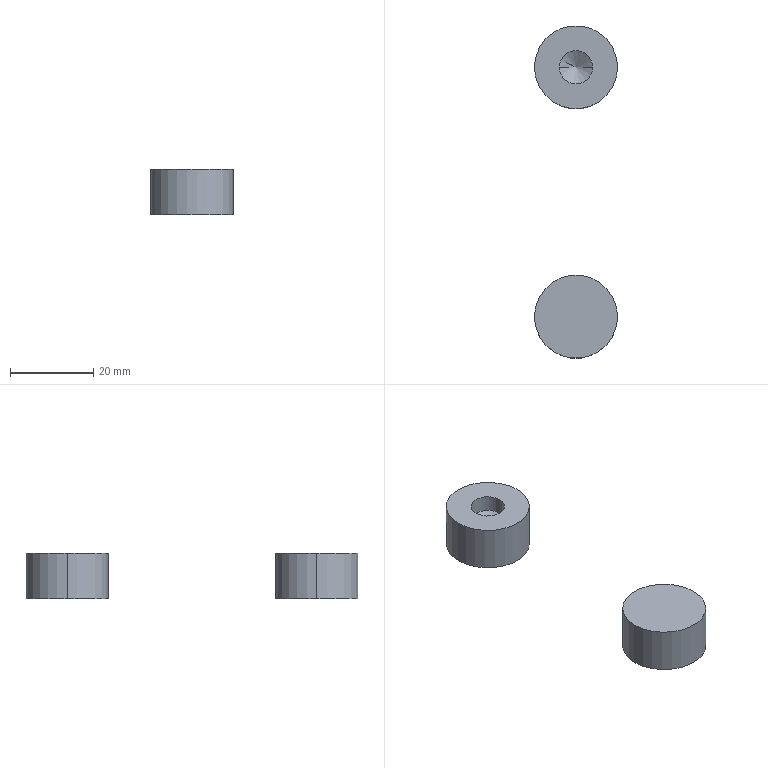Part | SolidWorks | features BaseBody 2 | 2 solids | 12 faces | box 20 x 80 x 11 mm | volume 6670 mm3 | cylinder 6 | plane 4 | cone 2 | commonest cylinder face diameters 20 x4 8 x2
STEP:
#1=CARTESIAN_POINT('',(70.,6.5,-439.5));
#2=VERTEX_POINT('',#1);
#3=CARTESIAN_POINT('',(50.,6.5,-439.5));
#4=VERTEX_POINT('',#3);
#5=CARTESIAN_POINT('',(60.,6.5,-439.5));
#6=DIRECTION('',(0.,0.,1.));
#7=DIRECTION('',(-1.,0.,0.));
#8=AXIS2_PLACEMENT_3D('',#5,#6,#7);
#9=CIRCLE('',#8,10.);
#10=EDGE_CURVE('',#2,#4,#9,.T.);
#11=ORIENTED_EDGE('',*,*,#10,.T.);
#12=CARTESIAN_POINT('',(50.,6.5,-428.5));
#13=VERTEX_POINT('',#12);
#14=CARTESIAN_POINT('',(50.,6.5,-439.5));
#15=DIRECTION('',(0.,0.,1.));
#16=VECTOR('',#15,1000.);
#17=LINE('',#14,#16);
#18=EDGE_CURVE('',#4,#13,#17,.T.);
#19=ORIENTED_EDGE('',*,*,#18,.T.);
#20=CARTESIAN_POINT('',(70.,6.5,-428.5));
#21=VERTEX_POINT('',#20);
#22=CARTESIAN_POINT('',(60.,6.5,-428.5));
#23=DIRECTION('',(0.,0.,1.));
#24=DIRECTION('',(-1.,0.,0.));
#25=AXIS2_PLACEMENT_3D('',#22,#23,#24);
#26=CIRCLE('',#25,10.);
#27=EDGE_CURVE('',#21,#13,#26,.T.);
#28=ORIENTED_EDGE('',*,*,#27,.F.);
#29=CARTESIAN_POINT('',(70.,6.5,-439.5));
#30=DIRECTION('',(0.,0.,1.));
#31=VECTOR('',#30,1000.);
#32=LINE('',#29,#31);
#33=EDGE_CURVE('',#2,#21,#32,.T.);
#34=ORIENTED_EDGE('',*,*,#33,.F.);
#35=EDGE_LOOP('',(#11,#19,#28,#34));
#36=FACE_OUTER_BOUND('',#35,.T.);
#37=CARTESIAN_POINT('',(60.,6.5,-439.5));
#38=DIRECTION('',(0.,0.,1.));
#39=DIRECTION('',(1.,0.,0.));
#40=AXIS2_PLACEMENT_3D('',#37,#38,#39);
#41=CYLINDRICAL_SURFACE('',#40,10.);
#42=ADVANCED_FACE('',(#36),#41,.T.);
#43=ORIENTED_EDGE('',*,*,#27,.T.);
#44=CARTESIAN_POINT('',(60.,6.5,-428.5));
#45=DIRECTION('',(0.,0.,1.));
#46=DIRECTION('',(-1.,0.,0.));
#47=AXIS2_PLACEMENT_3D('',#44,#45,#46);
#48=CIRCLE('',#47,10.);
#49=EDGE_CURVE('',#13,#21,#48,.T.);
#50=ORIENTED_EDGE('',*,*,#49,.T.);
#51=EDGE_LOOP('',(#43,#50));
#52=FACE_OUTER_BOUND('',#51,.T.);
#53=CARTESIAN_POINT('',(60.,6.5,-428.5));
#54=DIRECTION('',(0.,0.,-1.));
#55=DIRECTION('',(0.,-1.,0.));
#56=AXIS2_PLACEMENT_3D('',#53,#54,#55);
#57=PLANE('',#56);
#58=ADVANCED_FACE('',(#52),#57,.F.);
#59=ORIENTED_EDGE('',*,*,#10,.F.);
#60=CARTESIAN_POINT('',(60.,6.5,-439.5));
#61=DIRECTION('',(0.,0.,1.));
#62=DIRECTION('',(-1.,0.,0.));
#63=AXIS2_PLACEMENT_3D('',#60,#61,#62);
#64=CIRCLE('',#63,10.);
#65=EDGE_CURVE('',#4,#2,#64,.T.);
#66=ORIENTED_EDGE('',*,*,#65,.F.);
#67=EDGE_LOOP('',(#59,#66));
#68=FACE_OUTER_BOUND('',#67,.T.);
#69=CARTESIAN_POINT('',(60.,6.5,-439.5));
#70=DIRECTION('',(0.,0.,-1.));
#71=DIRECTION('',(0.,-1.,0.));
#72=AXIS2_PLACEMENT_3D('',#69,#70,#71);
#73=PLANE('',#72);
#74=ADVANCED_FACE('',(#68),#73,.T.);
#75=ORIENTED_EDGE('',*,*,#18,.F.);
#76=ORIENTED_EDGE('',*,*,#65,.T.);
#77=ORIENTED_EDGE('',*,*,#33,.T.);
#78=ORIENTED_EDGE('',*,*,#49,.F.);
#79=EDGE_LOOP('',(#75,#76,#77,#78));
#80=FACE_OUTER_BOUND('',#79,.T.);
#81=CARTESIAN_POINT('',(60.,6.5,-439.5));
#82=DIRECTION('',(0.,0.,1.));
#83=DIRECTION('',(1.,0.,0.));
#84=AXIS2_PLACEMENT_3D('',#81,#82,#83);
#85=CYLINDRICAL_SURFACE('',#84,10.);
#86=ADVANCED_FACE('',(#80),#85,.T.);
#87=CLOSED_SHELL('',(#42,#58,#74,#86));
#88=MANIFOLD_SOLID_BREP('',#87);
#89=CARTESIAN_POINT('',(50.,66.5,-439.5));
#90=VERTEX_POINT('',#89);
#91=CARTESIAN_POINT('',(70.,66.5,-439.5));
#92=VERTEX_POINT('',#91);
#93=CARTESIAN_POINT('',(60.,66.5,-439.5));
#94=DIRECTION('',(0.,0.,-1.));
#95=DIRECTION('',(-1.,0.,0.));
#96=AXIS2_PLACEMENT_3D('',#93,#94,#95);
#97=CIRCLE('',#96,10.);
#98=EDGE_CURVE('',#90,#92,#97,.T.);
#99=ORIENTED_EDGE('',*,*,#98,.F.);
#100=CARTESIAN_POINT('',(50.,66.5,-428.5));
#101=VERTEX_POINT('',#100);
#102=CARTESIAN_POINT('',(50.,66.5,-439.5));
#103=DIRECTION('',(0.,0.,1.));
#104=VECTOR('',#103,1000.);
#105=LINE('',#102,#104);
#106=EDGE_CURVE('',#90,#101,#105,.T.);
#107=ORIENTED_EDGE('',*,*,#106,.T.);
#108=CARTESIAN_POINT('',(70.,66.5,-428.5));
#109=VERTEX_POINT('',#108);
#110=CARTESIAN_POINT('',(60.,66.5,-428.5));
#111=DIRECTION('',(0.,0.,-1.));
#112=DIRECTION('',(-1.,0.,0.));
#113=AXIS2_PLACEMENT_3D('',#110,#111,#112);
#114=CIRCLE('',#113,10.);
#115=EDGE_CURVE('',#101,#109,#114,.T.);
#116=ORIENTED_EDGE('',*,*,#115,.T.);
#117=CARTESIAN_POINT('',(70.,66.5,-439.5));
#118=DIRECTION('',(0.,0.,1.));
#119=VECTOR('',#118,1000.);
#120=LINE('',#117,#119);
#121=EDGE_CURVE('',#92,#109,#120,.T.);
#122=ORIENTED_EDGE('',*,*,#121,.F.);
#123=EDGE_LOOP('',(#99,#107,#116,#122));
#124=FACE_OUTER_BOUND('',#123,.T.);
#125=CARTESIAN_POINT('',(60.,66.5,-439.5));
#126=DIRECTION('',(0.,0.,1.));
#127=DIRECTION('',(1.,0.,0.));
#128=AXIS2_PLACEMENT_3D('',#125,#126,#127);
#129=CYLINDRICAL_SURFACE('',#128,10.);
#130=ADVANCED_FACE('',(#124),#129,.T.);
#131=CARTESIAN_POINT('',(60.,66.5,-434.903));
#132=VERTEX_POINT('',#131);
#133=CARTESIAN_POINT('',(64.,66.5,-432.5));
#134=VERTEX_POINT('',#133);
#135=CARTESIAN_POINT('',(64.,66.5,-432.5));
#136=DIRECTION('',(0.8572,0.,0.515));
#137=VECTOR('',#136,1000.);
#138=LINE('',#135,#137);
#139=EDGE_CURVE('',#132,#134,#138,.T.);
#140=ORIENTED_EDGE('',*,*,#139,.F.);
#141=CARTESIAN_POINT('',(56.,66.5,-432.5));
#142=VERTEX_POINT('',#141);
#143=CARTESIAN_POINT('',(56.,66.5,-432.5));
#144=DIRECTION('',(-0.8572,0.,0.515));
#145=VECTOR('',#144,1000.);
#146=LINE('',#143,#145);
#147=EDGE_CURVE('',#132,#142,#146,.T.);
#148=ORIENTED_EDGE('',*,*,#147,.T.);
#149=CARTESIAN_POINT('',(60.,66.5,-432.5));
#150=DIRECTION('',(0.,0.,1.));
#151=DIRECTION('',(-1.,0.,0.));
#152=AXIS2_PLACEMENT_3D('',#149,#150,#151);
#153=CIRCLE('',#152,4.);
#154=EDGE_CURVE('',#142,#134,#153,.T.);
#155=ORIENTED_EDGE('',*,*,#154,.T.);
#156=EDGE_LOOP('',(#140,#148,#155));
#157=FACE_OUTER_BOUND('',#156,.T.);
#158=CARTESIAN_POINT('',(60.,66.5,-432.5));
#159=DIRECTION('',(0.,0.,1.));
#160=DIRECTION('',(1.,0.,0.));
#161=AXIS2_PLACEMENT_3D('',#158,#159,#160);
#162=CONICAL_SURFACE('',#161,4.,1.03);
#163=ADVANCED_FACE('',(#157),#162,.F.);
#164=CARTESIAN_POINT('',(64.,66.5,-428.5));
#165=VERTEX_POINT('',#164);
#166=CARTESIAN_POINT('',(56.,66.5,-428.5));
#167=VERTEX_POINT('',#166);
#168=CARTESIAN_POINT('',(60.,66.5,-428.5));
#169=DIRECTION('',(0.,0.,-1.));
#170=DIRECTION('',(-1.,0.,0.));
#171=AXIS2_PLACEMENT_3D('',#168,#169,#170);
#172=CIRCLE('',#171,4.);
#173=EDGE_CURVE('',#165,#167,#172,.T.);
#174=ORIENTED_EDGE('',*,*,#173,.F.);
#175=CARTESIAN_POINT('',(64.,66.5,-428.5));
#176=DIRECTION('',(0.,0.,-1.));
#177=VECTOR('',#176,1000.);
#178=LINE('',#175,#177);
#179=EDGE_CURVE('',#165,#134,#178,.T.);
#180=ORIENTED_EDGE('',*,*,#179,.T.);
#181=ORIENTED_EDGE('',*,*,#154,.F.);
#182=CARTESIAN_POINT('',(56.,66.5,-428.5));
#183=DIRECTION('',(0.,0.,-1.));
#184=VECTOR('',#183,1000.);
#185=LINE('',#182,#184);
#186=EDGE_CURVE('',#167,#142,#185,.T.);
#187=ORIENTED_EDGE('',*,*,#186,.F.);
#188=EDGE_LOOP('',(#174,#180,#181,#187));
#189=FACE_OUTER_BOUND('',#188,.T.);
#190=CARTESIAN_POINT('',(60.,66.5,-428.5));
#191=DIRECTION('',(0.,0.,-1.));
#192=DIRECTION('',(-1.,0.,0.));
#193=AXIS2_PLACEMENT_3D('',#190,#191,#192);
#194=CYLINDRICAL_SURFACE('',#193,4.);
#195=ADVANCED_FACE('',(#189),#194,.F.);
#196=ORIENTED_EDGE('',*,*,#179,.F.);
#197=CARTESIAN_POINT('',(60.,66.5,-428.5));
#198=DIRECTION('',(0.,0.,-1.));
#199=DIRECTION('',(-1.,0.,0.));
#200=AXIS2_PLACEMENT_3D('',#197,#198,#199);
#201=CIRCLE('',#200,4.);
#202=EDGE_CURVE('',#167,#165,#201,.T.);
#203=ORIENTED_EDGE('',*,*,#202,.F.);
#204=ORIENTED_EDGE('',*,*,#186,.T.);
#205=CARTESIAN_POINT('',(60.,66.5,-432.5));
#206=DIRECTION('',(0.,0.,1.));
#207=DIRECTION('',(-1.,0.,0.));
#208=AXIS2_PLACEMENT_3D('',#205,#206,#207);
#209=CIRCLE('',#208,4.);
#210=EDGE_CURVE('',#134,#142,#209,.T.);
#211=ORIENTED_EDGE('',*,*,#210,.F.);
#212=EDGE_LOOP('',(#196,#203,#204,#211));
#213=FACE_OUTER_BOUND('',#212,.T.);
#214=CARTESIAN_POINT('',(60.,66.5,-428.5));
#215=DIRECTION('',(0.,0.,-1.));
#216=DIRECTION('',(-1.,0.,0.));
#217=AXIS2_PLACEMENT_3D('',#214,#215,#216);
#218=CYLINDRICAL_SURFACE('',#217,4.);
#219=ADVANCED_FACE('',(#213),#218,.F.);
#220=ORIENTED_EDGE('',*,*,#147,.F.);
#221=ORIENTED_EDGE('',*,*,#139,.T.);
#222=ORIENTED_EDGE('',*,*,#210,.T.);
#223=EDGE_LOOP('',(#220,#221,#222));
#224=FACE_OUTER_BOUND('',#223,.T.);
#225=CARTESIAN_POINT('',(60.,66.5,-432.5));
#226=DIRECTION('',(0.,0.,1.));
#227=DIRECTION('',(1.,0.,0.));
#228=AXIS2_PLACEMENT_3D('',#225,#226,#227);
#229=CONICAL_SURFACE('',#228,4.,1.03);
#230=ADVANCED_FACE('',(#224),#229,.F.);
#231=CARTESIAN_POINT('',(60.,66.5,-428.5));
#232=DIRECTION('',(0.,0.,-1.));
#233=DIRECTION('',(-1.,0.,0.));
#234=AXIS2_PLACEMENT_3D('',#231,#232,#233);
#235=CIRCLE('',#234,10.);
#236=EDGE_CURVE('',#109,#101,#235,.T.);
#237=ORIENTED_EDGE('',*,*,#236,.F.);
#238=ORIENTED_EDGE('',*,*,#115,.F.);
#239=EDGE_LOOP('',(#237,#238));
#240=FACE_OUTER_BOUND('',#239,.T.);
#241=ORIENTED_EDGE('',*,*,#202,.T.);
#242=ORIENTED_EDGE('',*,*,#173,.T.);
#243=EDGE_LOOP('',(#241,#242));
#244=FACE_BOUND('',#243,.T.);
#245=CARTESIAN_POINT('',(60.,66.5,-428.5));
#246=DIRECTION('',(0.,0.,1.));
#247=DIRECTION('',(1.,0.,0.));
#248=AXIS2_PLACEMENT_3D('',#245,#246,#247);
#249=PLANE('',#248);
#250=ADVANCED_FACE('',(#240,#244),#249,.T.);
#251=CARTESIAN_POINT('',(60.,66.5,-439.5));
#252=DIRECTION('',(0.,0.,-1.));
#253=DIRECTION('',(-1.,0.,0.));
#254=AXIS2_PLACEMENT_3D('',#251,#252,#253);
#255=CIRCLE('',#254,10.);
#256=EDGE_CURVE('',#92,#90,#255,.T.);
#257=ORIENTED_EDGE('',*,*,#256,.T.);
#258=ORIENTED_EDGE('',*,*,#98,.T.);
#259=EDGE_LOOP('',(#257,#258));
#260=FACE_OUTER_BOUND('',#259,.T.);
#261=CARTESIAN_POINT('',(60.,66.5,-439.5));
#262=DIRECTION('',(0.,0.,1.));
#263=DIRECTION('',(1.,0.,0.));
#264=AXIS2_PLACEMENT_3D('',#261,#262,#263);
#265=PLANE('',#264);
#266=ADVANCED_FACE('',(#260),#265,.F.);
#267=ORIENTED_EDGE('',*,*,#106,.F.);
#268=ORIENTED_EDGE('',*,*,#256,.F.);
#269=ORIENTED_EDGE('',*,*,#121,.T.);
#270=ORIENTED_EDGE('',*,*,#236,.T.);
#271=EDGE_LOOP('',(#267,#268,#269,#270));
#272=FACE_OUTER_BOUND('',#271,.T.);
#273=CARTESIAN_POINT('',(60.,66.5,-439.5));
#274=DIRECTION('',(0.,0.,1.));
#275=DIRECTION('',(1.,0.,0.));
#276=AXIS2_PLACEMENT_3D('',#273,#274,#275);
#277=CYLINDRICAL_SURFACE('',#276,10.);
#278=ADVANCED_FACE('',(#272),#277,.T.);
#279=CLOSED_SHELL('',(#130,#163,#195,#219,#230,#250,#266,#278));
#280=MANIFOLD_SOLID_BREP('',#279);
#281=CARTESIAN_POINT('',(0.,0.,0.));
#282=DIRECTION('',(0.,0.,1.));
#283=DIRECTION('',(1.,0.,0.));
#284=AXIS2_PLACEMENT_3D('',#281,#282,#283);
#285=(LENGTH_UNIT()NAMED_UNIT(*)SI_UNIT(.MILLI.,.METRE.));
#286=UNCERTAINTY_MEASURE_WITH_UNIT(LENGTH_MEASURE(0.00001),#285,'','');
#287=(NAMED_UNIT(*)PLANE_ANGLE_UNIT()SI_UNIT($,.RADIAN.));
#288=(NAMED_UNIT(*)SI_UNIT($,.STERADIAN.)SOLID_ANGLE_UNIT());
#289=(GEOMETRIC_REPRESENTATION_CONTEXT(3)GLOBAL_UNCERTAINTY_ASSIGNED_CONTEXT((#286))GLOBAL_UNIT_ASSIGNED_CONTEXT((#285,#287,#288))REPRESENTATION_CONTEXT('',''));
#290=ADVANCED_BREP_SHAPE_REPRESENTATION('',(#88,#280,#284),#289);